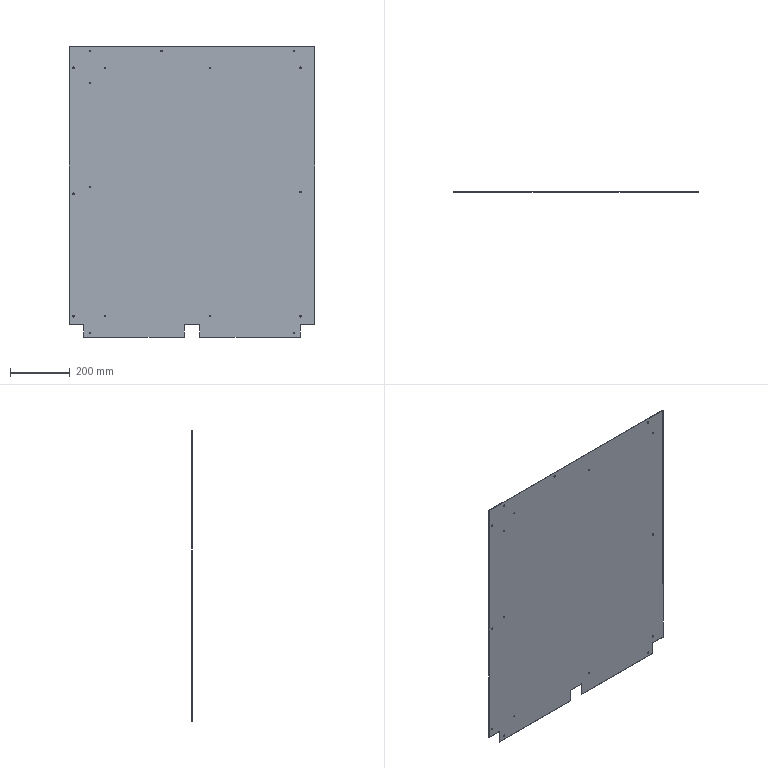Part | NX | features BREP 1 | 1 solid | 48 faces | box 821 x 1.5 x 971 mm | volume 1185775 mm3 | cylinder 34 | plane 14 | commonest cylinder face diameters 5 x22 3.3 x12